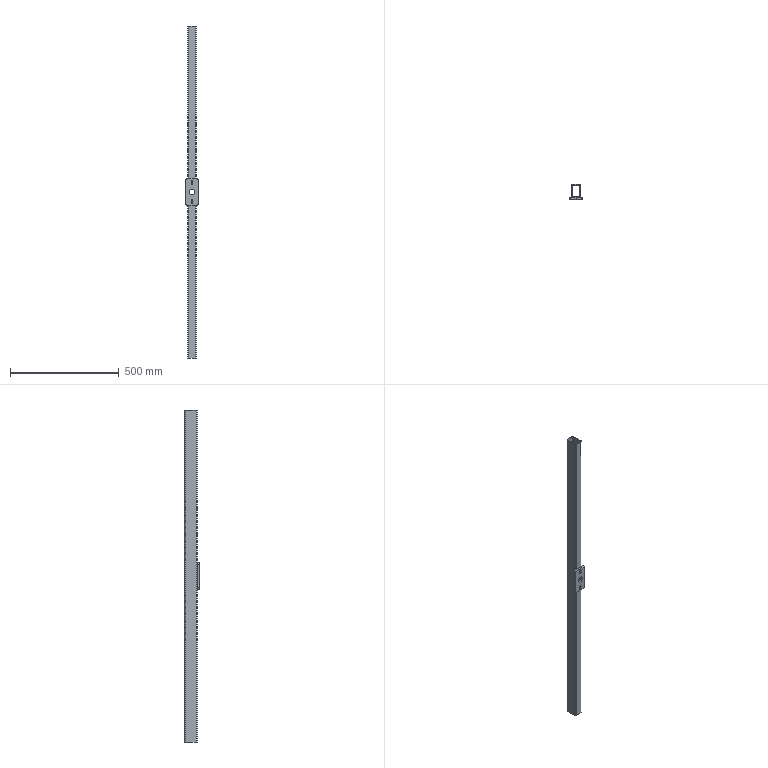Part | SolidWorks | features ICE 3, Fillet 1, WeldMemberFeat 1, WeldmentFeature 1 | 2 solids | 52 faces | box 60 x 70 x 1530 mm | volume 886735 mm3 | cylinder 32 | plane 20 | commonest cylinder face diameters 10 x12 9 x6 26 x6 6 x4 12 x4